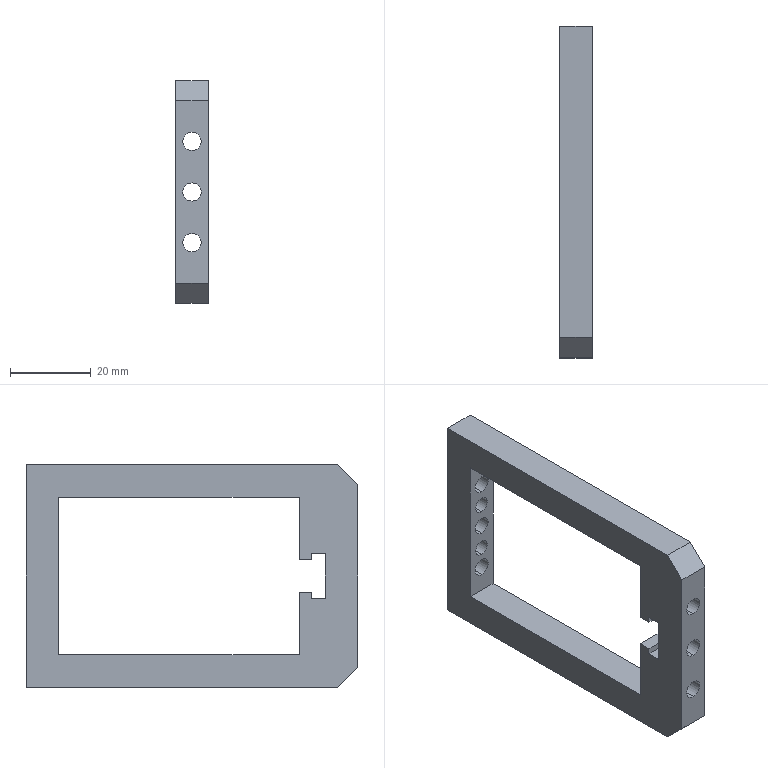Part | STEP file | 11-FG-B02211 | 1 solid | 36 faces | box 8 x 82 x 55 mm | volume 15645 mm3 | plane 20 | cylinder 16 | commonest cylinder face diameters 4.5 x12 4 x4
STEP:
#1=CARTESIAN_POINT('',(4.,74.,31.75));
#2=VERTEX_POINT('',#1);
#3=CARTESIAN_POINT('',(4.,74.,35.75));
#4=VERTEX_POINT('',#3);
#5=CARTESIAN_POINT('',(4.,74.,33.75));
#6=DIRECTION('',(0.,1.,0.));
#7=DIRECTION('',(0.,0.,1.));
#8=AXIS2_PLACEMENT_3D('',#5,#6,#7);
#9=CIRCLE('',#8,2.);
#10=EDGE_CURVE('',#2,#4,#9,.T.);
#11=ORIENTED_EDGE('',*,*,#10,.F.);
#12=CARTESIAN_POINT('',(4.,82.,31.75));
#13=VERTEX_POINT('',#12);
#14=CARTESIAN_POINT('',(4.,72.,31.75));
#15=DIRECTION('',(0.,1.,0.));
#16=VECTOR('',#15,1000.);
#17=LINE('',#14,#16);
#18=EDGE_CURVE('',#2,#13,#17,.T.);
#19=ORIENTED_EDGE('',*,*,#18,.T.);
#20=CARTESIAN_POINT('',(4.,82.,35.75));
#21=VERTEX_POINT('',#20);
#22=CARTESIAN_POINT('',(4.,82.,33.75));
#23=DIRECTION('',(0.,1.,0.));
#24=DIRECTION('',(0.,0.,1.));
#25=AXIS2_PLACEMENT_3D('',#22,#23,#24);
#26=CIRCLE('',#25,2.);
#27=EDGE_CURVE('',#13,#21,#26,.T.);
#28=ORIENTED_EDGE('',*,*,#27,.T.);
#29=CARTESIAN_POINT('',(4.,72.,35.75));
#30=DIRECTION('',(0.,1.,0.));
#31=VECTOR('',#30,1000.);
#32=LINE('',#29,#31);
#33=EDGE_CURVE('',#4,#21,#32,.T.);
#34=ORIENTED_EDGE('',*,*,#33,.F.);
#35=EDGE_LOOP('',(#11,#19,#28,#34));
#36=FACE_OUTER_BOUND('',#35,.T.);
#37=CARTESIAN_POINT('',(4.,72.,33.75));
#38=DIRECTION('',(0.,1.,0.));
#39=DIRECTION('',(0.,0.,1.));
#40=AXIS2_PLACEMENT_3D('',#37,#38,#39);
#41=CYLINDRICAL_SURFACE('',#40,2.);
#42=ADVANCED_FACE('',(#36),#41,.F.);
#43=CARTESIAN_POINT('',(4.,74.,18.839));
#44=VERTEX_POINT('',#43);
#45=CARTESIAN_POINT('',(4.,74.,22.839));
#46=VERTEX_POINT('',#45);
#47=CARTESIAN_POINT('',(4.,74.,20.839));
#48=DIRECTION('',(0.,1.,0.));
#49=DIRECTION('',(0.,0.,1.));
#50=AXIS2_PLACEMENT_3D('',#47,#48,#49);
#51=CIRCLE('',#50,2.);
#52=EDGE_CURVE('',#44,#46,#51,.T.);
#53=ORIENTED_EDGE('',*,*,#52,.F.);
#54=CARTESIAN_POINT('',(4.,82.,18.839));
#55=VERTEX_POINT('',#54);
#56=CARTESIAN_POINT('',(4.,72.,18.839));
#57=DIRECTION('',(0.,1.,0.));
#58=VECTOR('',#57,1000.);
#59=LINE('',#56,#58);
#60=EDGE_CURVE('',#44,#55,#59,.T.);
#61=ORIENTED_EDGE('',*,*,#60,.T.);
#62=CARTESIAN_POINT('',(4.,82.,22.839));
#63=VERTEX_POINT('',#62);
#64=CARTESIAN_POINT('',(4.,82.,20.839));
#65=DIRECTION('',(0.,1.,0.));
#66=DIRECTION('',(0.,0.,1.));
#67=AXIS2_PLACEMENT_3D('',#64,#65,#66);
#68=CIRCLE('',#67,2.);
#69=EDGE_CURVE('',#55,#63,#68,.T.);
#70=ORIENTED_EDGE('',*,*,#69,.T.);
#71=CARTESIAN_POINT('',(4.,72.,22.839));
#72=DIRECTION('',(0.,1.,0.));
#73=VECTOR('',#72,1000.);
#74=LINE('',#71,#73);
#75=EDGE_CURVE('',#46,#63,#74,.T.);
#76=ORIENTED_EDGE('',*,*,#75,.F.);
#77=EDGE_LOOP('',(#53,#61,#70,#76));
#78=FACE_OUTER_BOUND('',#77,.T.);
#79=CARTESIAN_POINT('',(4.,72.,20.839));
#80=DIRECTION('',(0.,1.,0.));
#81=DIRECTION('',(0.,0.,1.));
#82=AXIS2_PLACEMENT_3D('',#79,#80,#81);
#83=CYLINDRICAL_SURFACE('',#82,2.);
#84=ADVANCED_FACE('',(#78),#83,.F.);
#85=CARTESIAN_POINT('',(4.,74.,37.75));
#86=VERTEX_POINT('',#85);
#87=CARTESIAN_POINT('',(4.,74.,42.25));
#88=VERTEX_POINT('',#87);
#89=CARTESIAN_POINT('',(4.,74.,40.));
#90=DIRECTION('',(0.,1.,0.));
#91=DIRECTION('',(0.,0.,1.));
#92=AXIS2_PLACEMENT_3D('',#89,#90,#91);
#93=CIRCLE('',#92,2.25);
#94=EDGE_CURVE('',#86,#88,#93,.T.);
#95=ORIENTED_EDGE('',*,*,#94,.F.);
#96=CARTESIAN_POINT('',(4.,82.,37.75));
#97=VERTEX_POINT('',#96);
#98=CARTESIAN_POINT('',(4.,0.,37.75));
#99=DIRECTION('',(0.,1.,0.));
#100=VECTOR('',#99,1000.);
#101=LINE('',#98,#100);
#102=EDGE_CURVE('',#86,#97,#101,.T.);
#103=ORIENTED_EDGE('',*,*,#102,.T.);
#104=CARTESIAN_POINT('',(4.,82.,42.25));
#105=VERTEX_POINT('',#104);
#106=CARTESIAN_POINT('',(4.,82.,40.));
#107=DIRECTION('',(0.,1.,0.));
#108=DIRECTION('',(0.,0.,1.));
#109=AXIS2_PLACEMENT_3D('',#106,#107,#108);
#110=CIRCLE('',#109,2.25);
#111=EDGE_CURVE('',#97,#105,#110,.T.);
#112=ORIENTED_EDGE('',*,*,#111,.T.);
#113=CARTESIAN_POINT('',(4.,0.,42.25));
#114=DIRECTION('',(0.,1.,0.));
#115=VECTOR('',#114,1000.);
#116=LINE('',#113,#115);
#117=EDGE_CURVE('',#88,#105,#116,.T.);
#118=ORIENTED_EDGE('',*,*,#117,.F.);
#119=EDGE_LOOP('',(#95,#103,#112,#118));
#120=FACE_OUTER_BOUND('',#119,.T.);
#121=CARTESIAN_POINT('',(4.,0.,40.));
#122=DIRECTION('',(0.,1.,0.));
#123=DIRECTION('',(0.,0.,1.));
#124=AXIS2_PLACEMENT_3D('',#121,#122,#123);
#125=CYLINDRICAL_SURFACE('',#124,2.25);
#126=ADVANCED_FACE('',(#120),#125,.F.);
#127=CARTESIAN_POINT('',(4.,0.,37.75));
#128=VERTEX_POINT('',#127);
#129=CARTESIAN_POINT('',(4.,0.,42.25));
#130=VERTEX_POINT('',#129);
#131=CARTESIAN_POINT('',(4.,0.,40.));
#132=DIRECTION('',(0.,1.,0.));
#133=DIRECTION('',(0.,0.,1.));
#134=AXIS2_PLACEMENT_3D('',#131,#132,#133);
#135=CIRCLE('',#134,2.25);
#136=EDGE_CURVE('',#128,#130,#135,.T.);
#137=ORIENTED_EDGE('',*,*,#136,.F.);
#138=CARTESIAN_POINT('',(4.,14.5,37.75));
#139=VERTEX_POINT('',#138);
#140=CARTESIAN_POINT('',(4.,0.,37.75));
#141=DIRECTION('',(0.,1.,0.));
#142=VECTOR('',#141,1000.);
#143=LINE('',#140,#142);
#144=EDGE_CURVE('',#128,#139,#143,.T.);
#145=ORIENTED_EDGE('',*,*,#144,.T.);
#146=CARTESIAN_POINT('',(4.,14.5,42.25));
#147=VERTEX_POINT('',#146);
#148=CARTESIAN_POINT('',(4.,14.5,40.));
#149=DIRECTION('',(0.,1.,0.));
#150=DIRECTION('',(0.,0.,1.));
#151=AXIS2_PLACEMENT_3D('',#148,#149,#150);
#152=CIRCLE('',#151,2.25);
#153=EDGE_CURVE('',#139,#147,#152,.T.);
#154=ORIENTED_EDGE('',*,*,#153,.T.);
#155=CARTESIAN_POINT('',(4.,0.,42.25));
#156=DIRECTION('',(0.,1.,0.));
#157=VECTOR('',#156,1000.);
#158=LINE('',#155,#157);
#159=EDGE_CURVE('',#130,#147,#158,.T.);
#160=ORIENTED_EDGE('',*,*,#159,.F.);
#161=EDGE_LOOP('',(#137,#145,#154,#160));
#162=FACE_OUTER_BOUND('',#161,.T.);
#163=CARTESIAN_POINT('',(4.,0.,40.));
#164=DIRECTION('',(0.,1.,0.));
#165=DIRECTION('',(0.,0.,1.));
#166=AXIS2_PLACEMENT_3D('',#163,#164,#165);
#167=CYLINDRICAL_SURFACE('',#166,2.25);
#168=ADVANCED_FACE('',(#162),#167,.F.);
#169=CARTESIAN_POINT('',(4.,74.,25.25));
#170=VERTEX_POINT('',#169);
#171=CARTESIAN_POINT('',(4.,74.,29.75));
#172=VERTEX_POINT('',#171);
#173=CARTESIAN_POINT('',(4.,74.,27.5));
#174=DIRECTION('',(0.,1.,0.));
#175=DIRECTION('',(0.,0.,1.));
#176=AXIS2_PLACEMENT_3D('',#173,#174,#175);
#177=CIRCLE('',#176,2.25);
#178=EDGE_CURVE('',#170,#172,#177,.T.);
#179=ORIENTED_EDGE('',*,*,#178,.F.);
#180=CARTESIAN_POINT('',(4.,82.,25.25));
#181=VERTEX_POINT('',#180);
#182=CARTESIAN_POINT('',(4.,0.,25.25));
#183=DIRECTION('',(0.,1.,0.));
#184=VECTOR('',#183,1000.);
#185=LINE('',#182,#184);
#186=EDGE_CURVE('',#170,#181,#185,.T.);
#187=ORIENTED_EDGE('',*,*,#186,.T.);
#188=CARTESIAN_POINT('',(4.,82.,29.75));
#189=VERTEX_POINT('',#188);
#190=CARTESIAN_POINT('',(4.,82.,27.5));
#191=DIRECTION('',(0.,1.,0.));
#192=DIRECTION('',(0.,0.,1.));
#193=AXIS2_PLACEMENT_3D('',#190,#191,#192);
#194=CIRCLE('',#193,2.25);
#195=EDGE_CURVE('',#181,#189,#194,.T.);
#196=ORIENTED_EDGE('',*,*,#195,.T.);
#197=CARTESIAN_POINT('',(4.,0.,29.75));
#198=DIRECTION('',(0.,1.,0.));
#199=VECTOR('',#198,1000.);
#200=LINE('',#197,#199);
#201=EDGE_CURVE('',#172,#189,#200,.T.);
#202=ORIENTED_EDGE('',*,*,#201,.F.);
#203=EDGE_LOOP('',(#179,#187,#196,#202));
#204=FACE_OUTER_BOUND('',#203,.T.);
#205=CARTESIAN_POINT('',(4.,0.,27.5));
#206=DIRECTION('',(0.,1.,0.));
#207=DIRECTION('',(0.,0.,1.));
#208=AXIS2_PLACEMENT_3D('',#205,#206,#207);
#209=CYLINDRICAL_SURFACE('',#208,2.25);
#210=ADVANCED_FACE('',(#204),#209,.F.);
#211=CARTESIAN_POINT('',(4.,0.,25.25));
#212=VERTEX_POINT('',#211);
#213=CARTESIAN_POINT('',(4.,0.,29.75));
#214=VERTEX_POINT('',#213);
#215=CARTESIAN_POINT('',(4.,0.,27.5));
#216=DIRECTION('',(0.,1.,0.));
#217=DIRECTION('',(0.,0.,1.));
#218=AXIS2_PLACEMENT_3D('',#215,#216,#217);
#219=CIRCLE('',#218,2.25);
#220=EDGE_CURVE('',#212,#214,#219,.T.);
#221=ORIENTED_EDGE('',*,*,#220,.F.);
#222=CARTESIAN_POINT('',(4.,8.,25.25));
#223=VERTEX_POINT('',#222);
#224=CARTESIAN_POINT('',(4.,0.,25.25));
#225=DIRECTION('',(0.,1.,0.));
#226=VECTOR('',#225,1000.);
#227=LINE('',#224,#226);
#228=EDGE_CURVE('',#212,#223,#227,.T.);
#229=ORIENTED_EDGE('',*,*,#228,.T.);
#230=CARTESIAN_POINT('',(4.,8.,29.75));
#231=VERTEX_POINT('',#230);
#232=CARTESIAN_POINT('',(4.,8.,27.5));
#233=DIRECTION('',(0.,-1.,0.));
#234=DIRECTION('',(0.,0.,-1.));
#235=AXIS2_PLACEMENT_3D('',#232,#233,#234);
#236=CIRCLE('',#235,2.25);
#237=EDGE_CURVE('',#231,#223,#236,.T.);
#238=ORIENTED_EDGE('',*,*,#237,.F.);
#239=CARTESIAN_POINT('',(4.,0.,29.75));
#240=DIRECTION('',(0.,1.,0.));
#241=VECTOR('',#240,1000.);
#242=LINE('',#239,#241);
#243=EDGE_CURVE('',#214,#231,#242,.T.);
#244=ORIENTED_EDGE('',*,*,#243,.F.);
#245=EDGE_LOOP('',(#221,#229,#238,#244));
#246=FACE_OUTER_BOUND('',#245,.T.);
#247=CARTESIAN_POINT('',(4.,0.,27.5));
#248=DIRECTION('',(0.,1.,0.));
#249=DIRECTION('',(0.,0.,1.));
#250=AXIS2_PLACEMENT_3D('',#247,#248,#249);
#251=CYLINDRICAL_SURFACE('',#250,2.25);
#252=ADVANCED_FACE('',(#246),#251,.F.);
#253=CARTESIAN_POINT('',(4.,74.,12.75));
#254=VERTEX_POINT('',#253);
#255=CARTESIAN_POINT('',(4.,74.,17.25));
#256=VERTEX_POINT('',#255);
#257=CARTESIAN_POINT('',(4.,74.,15.));
#258=DIRECTION('',(0.,1.,0.));
#259=DIRECTION('',(0.,0.,1.));
#260=AXIS2_PLACEMENT_3D('',#257,#258,#259);
#261=CIRCLE('',#260,2.25);
#262=EDGE_CURVE('',#254,#256,#261,.T.);
#263=ORIENTED_EDGE('',*,*,#262,.F.);
#264=CARTESIAN_POINT('',(4.,82.,12.75));
#265=VERTEX_POINT('',#264);
#266=CARTESIAN_POINT('',(4.,0.,12.75));
#267=DIRECTION('',(0.,1.,0.));
#268=VECTOR('',#267,1000.);
#269=LINE('',#266,#268);
#270=EDGE_CURVE('',#254,#265,#269,.T.);
#271=ORIENTED_EDGE('',*,*,#270,.T.);
#272=CARTESIAN_POINT('',(4.,82.,17.25));
#273=VERTEX_POINT('',#272);
#274=CARTESIAN_POINT('',(4.,82.,15.));
#275=DIRECTION('',(0.,1.,0.));
#276=DIRECTION('',(0.,0.,1.));
#277=AXIS2_PLACEMENT_3D('',#274,#275,#276);
#278=CIRCLE('',#277,2.25);
#279=EDGE_CURVE('',#265,#273,#278,.T.);
#280=ORIENTED_EDGE('',*,*,#279,.T.);
#281=CARTESIAN_POINT('',(4.,0.,17.25));
#282=DIRECTION('',(0.,1.,0.));
#283=VECTOR('',#282,1000.);
#284=LINE('',#281,#283);
#285=EDGE_CURVE('',#256,#273,#284,.T.);
#286=ORIENTED_EDGE('',*,*,#285,.F.);
#287=EDGE_LOOP('',(#263,#271,#280,#286));
#288=FACE_OUTER_BOUND('',#287,.T.);
#289=CARTESIAN_POINT('',(4.,0.,15.));
#290=DIRECTION('',(0.,1.,0.));
#291=DIRECTION('',(0.,0.,1.));
#292=AXIS2_PLACEMENT_3D('',#289,#290,#291);
#293=CYLINDRICAL_SURFACE('',#292,2.25);
#294=ADVANCED_FACE('',(#288),#293,.F.);
#295=CARTESIAN_POINT('',(4.,0.,12.75));
#296=VERTEX_POINT('',#295);
#297=CARTESIAN_POINT('',(4.,0.,17.25));
#298=VERTEX_POINT('',#297);
#299=CARTESIAN_POINT('',(4.,0.,15.));
#300=DIRECTION('',(0.,1.,0.));
#301=DIRECTION('',(0.,0.,1.));
#302=AXIS2_PLACEMENT_3D('',#299,#300,#301);
#303=CIRCLE('',#302,2.25);
#304=EDGE_CURVE('',#296,#298,#303,.T.);
#305=ORIENTED_EDGE('',*,*,#304,.F.);
#306=CARTESIAN_POINT('',(4.,14.5,12.75));
#307=VERTEX_POINT('',#306);
#308=CARTESIAN_POINT('',(4.,0.,12.75));
#309=DIRECTION('',(0.,1.,0.));
#310=VECTOR('',#309,1000.);
#311=LINE('',#308,#310);
#312=EDGE_CURVE('',#296,#307,#311,.T.);
#313=ORIENTED_EDGE('',*,*,#312,.T.);
#314=CARTESIAN_POINT('',(4.,14.5,17.25));
#315=VERTEX_POINT('',#314);
#316=CARTESIAN_POINT('',(4.,14.5,15.));
#317=DIRECTION('',(0.,1.,0.));
#318=DIRECTION('',(0.,0.,1.));
#319=AXIS2_PLACEMENT_3D('',#316,#317,#318);
#320=CIRCLE('',#319,2.25);
#321=EDGE_CURVE('',#307,#315,#320,.T.);
#322=ORIENTED_EDGE('',*,*,#321,.T.);
#323=CARTESIAN_POINT('',(4.,0.,17.25));
#324=DIRECTION('',(0.,1.,0.));
#325=VECTOR('',#324,1000.);
#326=LINE('',#323,#325);
#327=EDGE_CURVE('',#298,#315,#326,.T.);
#328=ORIENTED_EDGE('',*,*,#327,.F.);
#329=EDGE_LOOP('',(#305,#313,#322,#328));
#330=FACE_OUTER_BOUND('',#329,.T.);
#331=CARTESIAN_POINT('',(4.,0.,15.));
#332=DIRECTION('',(0.,1.,0.));
#333=DIRECTION('',(0.,0.,1.));
#334=AXIS2_PLACEMENT_3D('',#331,#332,#333);
#335=CYLINDRICAL_SURFACE('',#334,2.25);
#336=ADVANCED_FACE('',(#330),#335,.F.);
#337=CARTESIAN_POINT('',(0.,8.,22.));
#338=VERTEX_POINT('',#337);
#339=CARTESIAN_POINT('',(0.,8.,33.));
#340=VERTEX_POINT('',#339);
#341=CARTESIAN_POINT('',(0.,8.,8.));
#342=DIRECTION('',(0.,0.,1.));
#343=VECTOR('',#342,1000.);
#344=LINE('',#341,#343);
#345=EDGE_CURVE('',#338,#340,#344,.T.);
#346=ORIENTED_EDGE('',*,*,#345,.F.);
#347=CARTESIAN_POINT('',(0.,11.5,22.));
#348=VERTEX_POINT('',#347);
#349=CARTESIAN_POINT('',(0.,11.5,22.));
#350=DIRECTION('',(0.,1.,0.));
#351=VECTOR('',#350,1000.);
#352=LINE('',#349,#351);
#353=EDGE_CURVE('',#338,#348,#352,.T.);
#354=ORIENTED_EDGE('',*,*,#353,.T.);
#355=CARTESIAN_POINT('',(0.,11.5,23.5));
#356=VERTEX_POINT('',#355);
#357=CARTESIAN_POINT('',(0.,11.5,22.));
#358=DIRECTION('',(0.,0.,1.));
#359=VECTOR('',#358,1000.);
#360=LINE('',#357,#359);
#361=EDGE_CURVE('',#348,#356,#360,.T.);
#362=ORIENTED_EDGE('',*,*,#361,.T.);
#363=CARTESIAN_POINT('',(0.,14.5,23.5));
#364=VERTEX_POINT('',#363);
#365=CARTESIAN_POINT('',(0.,11.5,23.5));
#366=DIRECTION('',(0.,1.,0.));
#367=VECTOR('',#366,1000.);
#368=LINE('',#365,#367);
#369=EDGE_CURVE('',#356,#364,#368,.T.);
#370=ORIENTED_EDGE('',*,*,#369,.T.);
#371=CARTESIAN_POINT('',(0.,14.5,8.));
#372=VERTEX_POINT('',#371);
#373=CARTESIAN_POINT('',(0.,14.5,8.));
#374=DIRECTION('',(0.,0.,-1.));
#375=VECTOR('',#374,1000.);
#376=LINE('',#373,#375);
#377=EDGE_CURVE('',#364,#372,#376,.T.);
#378=ORIENTED_EDGE('',*,*,#377,.T.);
#379=CARTESIAN_POINT('',(0.,74.,8.));
#380=VERTEX_POINT('',#379);
#381=CARTESIAN_POINT('',(0.,74.,8.));
#382=DIRECTION('',(0.,-1.,0.));
#383=VECTOR('',#382,1000.);
#384=LINE('',#381,#383);
#385=EDGE_CURVE('',#380,#372,#384,.T.);
#386=ORIENTED_EDGE('',*,*,#385,.F.);
#387=CARTESIAN_POINT('',(0.,74.,47.));
#388=VERTEX_POINT('',#387);
#389=CARTESIAN_POINT('',(0.,74.,47.));
#390=DIRECTION('',(0.,0.,-1.));
#391=VECTOR('',#390,1000.);
#392=LINE('',#389,#391);
#393=EDGE_CURVE('',#388,#380,#392,.T.);
#394=ORIENTED_EDGE('',*,*,#393,.F.);
#395=CARTESIAN_POINT('',(0.,14.5,47.));
#396=VERTEX_POINT('',#395);
#397=CARTESIAN_POINT('',(0.,8.,47.));
#398=DIRECTION('',(0.,1.,0.));
#399=VECTOR('',#398,1000.);
#400=LINE('',#397,#399);
#401=EDGE_CURVE('',#396,#388,#400,.T.);
#402=ORIENTED_EDGE('',*,*,#401,.F.);
#403=CARTESIAN_POINT('',(0.,14.5,31.5));
#404=VERTEX_POINT('',#403);
#405=CARTESIAN_POINT('',(0.,14.5,31.5));
#406=DIRECTION('',(0.,0.,-1.));
#407=VECTOR('',#406,1000.);
#408=LINE('',#405,#407);
#409=EDGE_CURVE('',#396,#404,#408,.T.);
#410=ORIENTED_EDGE('',*,*,#409,.T.);
#411=CARTESIAN_POINT('',(0.,11.5,31.5));
#412=VERTEX_POINT('',#411);
#413=CARTESIAN_POINT('',(0.,11.5,31.5));
#414=DIRECTION('',(0.,-1.,0.));
#415=VECTOR('',#414,1000.);
#416=LINE('',#413,#415);
#417=EDGE_CURVE('',#404,#412,#416,.T.);
#418=ORIENTED_EDGE('',*,*,#417,.T.);
#419=CARTESIAN_POINT('',(0.,11.5,33.));
#420=VERTEX_POINT('',#419);
#421=CARTESIAN_POINT('',(0.,11.5,31.5));
#422=DIRECTION('',(0.,0.,1.));
#423=VECTOR('',#422,1000.);
#424=LINE('',#421,#423);
#425=EDGE_CURVE('',#412,#420,#424,.T.);
#426=ORIENTED_EDGE('',*,*,#425,.T.);
#427=CARTESIAN_POINT('',(0.,11.5,33.));
#428=DIRECTION('',(0.,-1.,0.));
#429=VECTOR('',#428,1000.);
#430=LINE('',#427,#429);
#431=EDGE_CURVE('',#420,#340,#430,.T.);
#432=ORIENTED_EDGE('',*,*,#431,.T.);
#433=EDGE_LOOP('',(#346,#354,#362,#370,#378,#386,#394,#402,#410,#418,#426,#432));
#434=FACE_BOUND('',#433,.T.);
#435=CARTESIAN_POINT('',(0.,82.,0.));
#436=VERTEX_POINT('',#435);
#437=CARTESIAN_POINT('',(0.,5.,0.));
#438=VERTEX_POINT('',#437);
#439=CARTESIAN_POINT('',(0.,0.,0.));
#440=DIRECTION('',(0.,-1.,0.));
#441=VECTOR('',#440,1000.);
#442=LINE('',#439,#441);
#443=EDGE_CURVE('',#436,#438,#442,.T.);
#444=ORIENTED_EDGE('',*,*,#443,.T.);
#445=CARTESIAN_POINT('',(0.,0.,5.));
#446=VERTEX_POINT('',#445);
#447=CARTESIAN_POINT('',(0.,0.,5.));
#448=DIRECTION('',(0.,-0.7071,0.7071));
#449=VECTOR('',#448,1000.);
#450=LINE('',#447,#449);
#451=EDGE_CURVE('',#438,#446,#450,.T.);
#452=ORIENTED_EDGE('',*,*,#451,.T.);
#453=CARTESIAN_POINT('',(0.,0.,50.));
#454=VERTEX_POINT('',#453);
#455=CARTESIAN_POINT('',(0.,0.,55.));
#456=DIRECTION('',(0.,0.,-1.));
#457=VECTOR('',#456,1000.);
#458=LINE('',#455,#457);
#459=EDGE_CURVE('',#454,#446,#458,.T.);
#460=ORIENTED_EDGE('',*,*,#459,.F.);
#461=CARTESIAN_POINT('',(0.,5.,55.));
#462=VERTEX_POINT('',#461);
#463=CARTESIAN_POINT('',(0.,5.,55.));
#464=DIRECTION('',(0.,0.7071,0.7071));
#465=VECTOR('',#464,1000.);
#466=LINE('',#463,#465);
#467=EDGE_CURVE('',#454,#462,#466,.T.);
#468=ORIENTED_EDGE('',*,*,#467,.T.);
#469=CARTESIAN_POINT('',(0.,82.,55.));
#470=VERTEX_POINT('',#469);
#471=CARTESIAN_POINT('',(0.,0.,55.));
#472=DIRECTION('',(0.,-1.,0.));
#473=VECTOR('',#472,1000.);
#474=LINE('',#471,#473);
#475=EDGE_CURVE('',#470,#462,#474,.T.);
#476=ORIENTED_EDGE('',*,*,#475,.F.);
#477=CARTESIAN_POINT('',(0.,82.,55.));
#478=DIRECTION('',(0.,0.,-1.));
#479=VECTOR('',#478,1000.);
#480=LINE('',#477,#479);
#481=EDGE_CURVE('',#470,#436,#480,.T.);
#482=ORIENTED_EDGE('',*,*,#481,.T.);
#483=EDGE_LOOP('',(#444,#452,#460,#468,#476,#482));
#484=FACE_OUTER_BOUND('',#483,.T.);
#485=CARTESIAN_POINT('',(0.,0.,55.));
#486=DIRECTION('',(1.,0.,0.));
#487=DIRECTION('',(0.,0.,-1.));
#488=AXIS2_PLACEMENT_3D('',#485,#486,#487);
#489=PLANE('',#488);
#490=ADVANCED_FACE('',(#434,#484),#489,.F.);
#491=CARTESIAN_POINT('',(4.,0.,40.));
#492=DIRECTION('',(0.,1.,0.));
#493=DIRECTION('',(0.,0.,1.));
#494=AXIS2_PLACEMENT_3D('',#491,#492,#493);
#495=CIRCLE('',#494,2.25);
#496=EDGE_CURVE('',#130,#128,#495,.T.);
#497=ORIENTED_EDGE('',*,*,#496,.T.);
#498=ORIENTED_EDGE('',*,*,#136,.T.);
#499=EDGE_LOOP('',(#497,#498));
#500=FACE_BOUND('',#499,.T.);
#501=CARTESIAN_POINT('',(4.,0.,27.5));
#502=DIRECTION('',(0.,1.,0.));
#503=DIRECTION('',(0.,0.,1.));
#504=AXIS2_PLACEMENT_3D('',#501,#502,#503);
#505=CIRCLE('',#504,2.25);
#506=EDGE_CURVE('',#214,#212,#505,.T.);
#507=ORIENTED_EDGE('',*,*,#506,.T.);
#508=ORIENTED_EDGE('',*,*,#220,.T.);
#509=EDGE_LOOP('',(#507,#508));
#510=FACE_BOUND('',#509,.T.);
#511=CARTESIAN_POINT('',(4.,0.,15.));
#512=DIRECTION('',(0.,1.,0.));
#513=DIRECTION('',(0.,0.,1.));
#514=AXIS2_PLACEMENT_3D('',#511,#512,#513);
#515=CIRCLE('',#514,2.25);
#516=EDGE_CURVE('',#298,#296,#515,.T.);
#517=ORIENTED_EDGE('',*,*,#516,.T.);
#518=ORIENTED_EDGE('',*,*,#304,.T.);
#519=EDGE_LOOP('',(#517,#518));
#520=FACE_BOUND('',#519,.T.);
#521=ORIENTED_EDGE('',*,*,#459,.T.);
#522=CARTESIAN_POINT('',(8.,0.,5.));
#523=VERTEX_POINT('',#522);
#524=CARTESIAN_POINT('',(8.,0.,5.));
#525=DIRECTION('',(1.,0.,0.));
#526=VECTOR('',#525,1000.);
#527=LINE('',#524,#526);
#528=EDGE_CURVE('',#446,#523,#527,.T.);
#529=ORIENTED_EDGE('',*,*,#528,.T.);
#530=CARTESIAN_POINT('',(8.,0.,50.));
#531=VERTEX_POINT('',#530);
#532=CARTESIAN_POINT('',(8.,0.,55.));
#533=DIRECTION('',(0.,0.,-1.));
#534=VECTOR('',#533,1000.);
#535=LINE('',#532,#534);
#536=EDGE_CURVE('',#531,#523,#535,.T.);
#537=ORIENTED_EDGE('',*,*,#536,.F.);
#538=CARTESIAN_POINT('',(0.,0.,50.));
#539=DIRECTION('',(-1.,0.,0.));
#540=VECTOR('',#539,1000.);
#541=LINE('',#538,#540);
#542=EDGE_CURVE('',#531,#454,#541,.T.);
#543=ORIENTED_EDGE('',*,*,#542,.T.);
#544=EDGE_LOOP('',(#521,#529,#537,#543));
#545=FACE_OUTER_BOUND('',#544,.T.);
#546=CARTESIAN_POINT('',(0.,0.,55.));
#547=DIRECTION('',(0.,1.,0.));
#548=DIRECTION('',(0.,0.,1.));
#549=AXIS2_PLACEMENT_3D('',#546,#547,#548);
#550=PLANE('',#549);
#551=ADVANCED_FACE('',(#500,#510,#520,#545),#550,.F.);
#552=CARTESIAN_POINT('',(8.,8.,22.));
#553=VERTEX_POINT('',#552);
#554=CARTESIAN_POINT('',(8.,11.5,22.));
#555=VERTEX_POINT('',#554);
#556=CARTESIAN_POINT('',(8.,11.5,22.));
#557=DIRECTION('',(0.,1.,0.));
#558=VECTOR('',#557,1000.);
#559=LINE('',#556,#558);
#560=EDGE_CURVE('',#553,#555,#559,.T.);
#561=ORIENTED_EDGE('',*,*,#560,.F.);
#562=CARTESIAN_POINT('',(8.,8.,33.));
#563=VERTEX_POINT('',#562);
#564=CARTESIAN_POINT('',(8.,8.,8.));
#565=DIRECTION('',(0.,0.,1.));
#566=VECTOR('',#565,1000.);
#567=LINE('',#564,#566);
#568=EDGE_CURVE('',#553,#563,#567,.T.);
#569=ORIENTED_EDGE('',*,*,#568,.T.);
#570=CARTESIAN_POINT('',(8.,11.5,33.));
#571=VERTEX_POINT('',#570);
#572=CARTESIAN_POINT('',(8.,11.5,33.));
#573=DIRECTION('',(0.,-1.,0.));
#574=VECTOR('',#573,1000.);
#575=LINE('',#572,#574);
#576=EDGE_CURVE('',#571,#563,#575,.T.);
#577=ORIENTED_EDGE('',*,*,#576,.F.);
#578=CARTESIAN_POINT('',(8.,11.5,31.5));
#579=VERTEX_POINT('',#578);
#580=CARTESIAN_POINT('',(8.,11.5,31.5));
#581=DIRECTION('',(0.,0.,1.));
#582=VECTOR('',#581,1000.);
#583=LINE('',#580,#582);
#584=EDGE_CURVE('',#579,#571,#583,.T.);
#585=ORIENTED_EDGE('',*,*,#584,.F.);
#586=CARTESIAN_POINT('',(8.,14.5,31.5));
#587=VERTEX_POINT('',#586);
#588=CARTESIAN_POINT('',(8.,11.5,31.5));
#589=DIRECTION('',(0.,-1.,0.));
#590=VECTOR('',#589,1000.);
#591=LINE('',#588,#590);
#592=EDGE_CURVE('',#587,#579,#591,.T.);
#593=ORIENTED_EDGE('',*,*,#592,.F.);
#594=CARTESIAN_POINT('',(8.,14.5,47.));
#595=VERTEX_POINT('',#594);
#596=CARTESIAN_POINT('',(8.,14.5,31.5));
#597=DIRECTION('',(0.,0.,-1.));
#598=VECTOR('',#597,1000.);
#599=LINE('',#596,#598);
#600=EDGE_CURVE('',#595,#587,#599,.T.);
#601=ORIENTED_EDGE('',*,*,#600,.F.);
#602=CARTESIAN_POINT('',(8.,74.,47.));
#603=VERTEX_POINT('',#602);
#604=CARTESIAN_POINT('',(8.,8.,47.));
#605=DIRECTION('',(0.,1.,0.));
#606=VECTOR('',#605,1000.);
#607=LINE('',#604,#606);
#608=EDGE_CURVE('',#595,#603,#607,.T.);
#609=ORIENTED_EDGE('',*,*,#608,.T.);
#610=CARTESIAN_POINT('',(8.,74.,8.));
#611=VERTEX_POINT('',#610);
#612=CARTESIAN_POINT('',(8.,74.,47.));
#613=DIRECTION('',(0.,0.,-1.));
#614=VECTOR('',#613,1000.);
#615=LINE('',#612,#614);
#616=EDGE_CURVE('',#603,#611,#615,.T.);
#617=ORIENTED_EDGE('',*,*,#616,.T.);
#618=CARTESIAN_POINT('',(8.,14.5,8.));
#619=VERTEX_POINT('',#618);
#620=CARTESIAN_POINT('',(8.,74.,8.));
#621=DIRECTION('',(0.,-1.,0.));
#622=VECTOR('',#621,1000.);
#623=LINE('',#620,#622);
#624=EDGE_CURVE('',#611,#619,#623,.T.);
#625=ORIENTED_EDGE('',*,*,#624,.T.);
#626=CARTESIAN_POINT('',(8.,14.5,23.5));
#627=VERTEX_POINT('',#626);
#628=CARTESIAN_POINT('',(8.,14.5,8.));
#629=DIRECTION('',(0.,0.,-1.));
#630=VECTOR('',#629,1000.);
#631=LINE('',#628,#630);
#632=EDGE_CURVE('',#627,#619,#631,.T.);
#633=ORIENTED_EDGE('',*,*,#632,.F.);
#634=CARTESIAN_POINT('',(8.,11.5,23.5));
#635=VERTEX_POINT('',#634);
#636=CARTESIAN_POINT('',(8.,11.5,23.5));
#637=DIRECTION('',(0.,1.,0.));
#638=VECTOR('',#637,1000.);
#639=LINE('',#636,#638);
#640=EDGE_CURVE('',#635,#627,#639,.T.);
#641=ORIENTED_EDGE('',*,*,#640,.F.);
#642=CARTESIAN_POINT('',(8.,11.5,22.));
#643=DIRECTION('',(0.,0.,1.));
#644=VECTOR('',#643,1000.);
#645=LINE('',#642,#644);
#646=EDGE_CURVE('',#555,#635,#645,.T.);
#647=ORIENTED_EDGE('',*,*,#646,.F.);
#648=EDGE_LOOP('',(#561,#569,#577,#585,#593,#601,#609,#617,#625,#633,#641,#647));
#649=FACE_BOUND('',#648,.T.);
#650=ORIENTED_EDGE('',*,*,#536,.T.);
#651=CARTESIAN_POINT('',(8.,5.,0.));
#652=VERTEX_POINT('',#651);
#653=CARTESIAN_POINT('',(8.,0.,5.));
#654=DIRECTION('',(0.,0.7071,-0.7071));
#655=VECTOR('',#654,1000.);
#656=LINE('',#653,#655);
#657=EDGE_CURVE('',#523,#652,#656,.T.);
#658=ORIENTED_EDGE('',*,*,#657,.T.);
#659=CARTESIAN_POINT('',(8.,82.,0.));
#660=VERTEX_POINT('',#659);
#661=CARTESIAN_POINT('',(8.,0.,0.));
#662=DIRECTION('',(0.,1.,0.));
#663=VECTOR('',#662,1000.);
#664=LINE('',#661,#663);
#665=EDGE_CURVE('',#652,#660,#664,.T.);
#666=ORIENTED_EDGE('',*,*,#665,.T.);
#667=CARTESIAN_POINT('',(8.,82.,55.));
#668=VERTEX_POINT('',#667);
#669=CARTESIAN_POINT('',(8.,82.,55.));
#670=DIRECTION('',(0.,0.,-1.));
#671=VECTOR('',#670,1000.);
#672=LINE('',#669,#671);
#673=EDGE_CURVE('',#668,#660,#672,.T.);
#674=ORIENTED_EDGE('',*,*,#673,.F.);
#675=CARTESIAN_POINT('',(8.,5.,55.));
#676=VERTEX_POINT('',#675);
#677=CARTESIAN_POINT('',(8.,0.,55.));
#678=DIRECTION('',(0.,1.,0.));
#679=VECTOR('',#678,1000.);
#680=LINE('',#677,#679);
#681=EDGE_CURVE('',#676,#668,#680,.T.);
#682=ORIENTED_EDGE('',*,*,#681,.F.);
#683=CARTESIAN_POINT('',(8.,5.,55.));
#684=DIRECTION('',(0.,-0.7071,-0.7071));
#685=VECTOR('',#684,1000.);
#686=LINE('',#683,#685);
#687=EDGE_CURVE('',#676,#531,#686,.T.);
#688=ORIENTED_EDGE('',*,*,#687,.T.);
#689=EDGE_LOOP('',(#650,#658,#666,#674,#682,#688));
#690=FACE_OUTER_BOUND('',#689,.T.);
#691=CARTESIAN_POINT('',(8.,0.,55.));
#692=DIRECTION('',(-1.,0.,0.));
#693=DIRECTION('',(0.,0.,1.));
#694=AXIS2_PLACEMENT_3D('',#691,#692,#693);
#695=PLANE('',#694);
#696=ADVANCED_FACE('',(#649,#690),#695,.F.);
#697=CARTESIAN_POINT('',(4.,82.,33.75));
#698=DIRECTION('',(0.,1.,0.));
#699=DIRECTION('',(0.,0.,1.));
#700=AXIS2_PLACEMENT_3D('',#697,#698,#699);
#701=CIRCLE('',#700,2.);
#702=EDGE_CURVE('',#21,#13,#701,.T.);
#703=ORIENTED_EDGE('',*,*,#702,.F.);
#704=ORIENTED_EDGE('',*,*,#27,.F.);
#705=EDGE_LOOP('',(#703,#704));
#706=FACE_BOUND('',#705,.T.);
#707=CARTESIAN_POINT('',(4.,82.,20.839));
#708=DIRECTION('',(0.,1.,0.));
#709=DIRECTION('',(0.,0.,1.));
#710=AXIS2_PLACEMENT_3D('',#707,#708,#709);
#711=CIRCLE('',#710,2.);
#712=EDGE_CURVE('',#63,#55,#711,.T.);
#713=ORIENTED_EDGE('',*,*,#712,.F.);
#714=ORIENTED_EDGE('',*,*,#69,.F.);
#715=EDGE_LOOP('',(#713,#714));
#716=FACE_BOUND('',#715,.T.);
#717=CARTESIAN_POINT('',(4.,82.,40.));
#718=DIRECTION('',(0.,1.,0.));
#719=DIRECTION('',(0.,0.,1.));
#720=AXIS2_PLACEMENT_3D('',#717,#718,#719);
#721=CIRCLE('',#720,2.25);
#722=EDGE_CURVE('',#105,#97,#721,.T.);
#723=ORIENTED_EDGE('',*,*,#722,.F.);
#724=ORIENTED_EDGE('',*,*,#111,.F.);
#725=EDGE_LOOP('',(#723,#724));
#726=FACE_BOUND('',#725,.T.);
#727=CARTESIAN_POINT('',(4.,82.,27.5));
#728=DIRECTION('',(0.,1.,0.));
#729=DIRECTION('',(0.,0.,1.));
#730=AXIS2_PLACEMENT_3D('',#727,#728,#729);
#731=CIRCLE('',#730,2.25);
#732=EDGE_CURVE('',#189,#181,#731,.T.);
#733=ORIENTED_EDGE('',*,*,#732,.F.);
#734=ORIENTED_EDGE('',*,*,#195,.F.);
#735=EDGE_LOOP('',(#733,#734));
#736=FACE_BOUND('',#735,.T.);
#737=CARTESIAN_POINT('',(4.,82.,15.));
#738=DIRECTION('',(0.,1.,0.));
#739=DIRECTION('',(0.,0.,1.));
#740=AXIS2_PLACEMENT_3D('',#737,#738,#739);
#741=CIRCLE('',#740,2.25);
#742=EDGE_CURVE('',#273,#265,#741,.T.);
#743=ORIENTED_EDGE('',*,*,#742,.F.);
#744=ORIENTED_EDGE('',*,*,#279,.F.);
#745=EDGE_LOOP('',(#743,#744));
#746=FACE_BOUND('',#745,.T.);
#747=CARTESIAN_POINT('',(0.,82.,0.));
#748=DIRECTION('',(-1.,0.,0.));
#749=VECTOR('',#748,1000.);
#750=LINE('',#747,#749);
#751=EDGE_CURVE('',#660,#436,#750,.T.);
#752=ORIENTED_EDGE('',*,*,#751,.T.);
#753=ORIENTED_EDGE('',*,*,#481,.F.);
#754=CARTESIAN_POINT('',(0.,82.,55.));
#755=DIRECTION('',(-1.,0.,0.));
#756=VECTOR('',#755,1000.);
#757=LINE('',#754,#756);
#758=EDGE_CURVE('',#668,#470,#757,.T.);
#759=ORIENTED_EDGE('',*,*,#758,.F.);
#760=ORIENTED_EDGE('',*,*,#673,.T.);
#761=EDGE_LOOP('',(#752,#753,#759,#760));
#762=FACE_OUTER_BOUND('',#761,.T.);
#763=CARTESIAN_POINT('',(0.,82.,55.));
#764=DIRECTION('',(0.,-1.,0.));
#765=DIRECTION('',(0.,0.,-1.));
#766=AXIS2_PLACEMENT_3D('',#763,#764,#765);
#767=PLANE('',#766);
#768=ADVANCED_FACE('',(#706,#716,#726,#736,#746,#762),#767,.F.);
#769=ORIENTED_EDGE('',*,*,#475,.T.);
#770=CARTESIAN_POINT('',(0.,5.,55.));
#771=DIRECTION('',(1.,0.,0.));
#772=VECTOR('',#771,1000.);
#773=LINE('',#770,#772);
#774=EDGE_CURVE('',#462,#676,#773,.T.);
#775=ORIENTED_EDGE('',*,*,#774,.T.);
#776=ORIENTED_EDGE('',*,*,#681,.T.);
#777=ORIENTED_EDGE('',*,*,#758,.T.);
#778=EDGE_LOOP('',(#769,#775,#776,#777));
#779=FACE_OUTER_BOUND('',#778,.T.);
#780=CARTESIAN_POINT('',(0.,82.,55.));
#781=DIRECTION('',(0.,0.,-1.));
#782=DIRECTION('',(-1.,0.,0.));
#783=AXIS2_PLACEMENT_3D('',#780,#781,#782);
#784=PLANE('',#783);
#785=ADVANCED_FACE('',(#779),#784,.F.);
#786=ORIENTED_EDGE('',*,*,#665,.F.);
#787=CARTESIAN_POINT('',(0.,5.,0.));
#788=DIRECTION('',(-1.,0.,0.));
#789=VECTOR('',#788,1000.);
#790=LINE('',#787,#789);
#791=EDGE_CURVE('',#652,#438,#790,.T.);
#792=ORIENTED_EDGE('',*,*,#791,.T.);
#793=ORIENTED_EDGE('',*,*,#443,.F.);
#794=ORIENTED_EDGE('',*,*,#751,.F.);
#795=EDGE_LOOP('',(#786,#792,#793,#794));
#796=FACE_OUTER_BOUND('',#795,.T.);
#797=CARTESIAN_POINT('',(0.,82.,0.));
#798=DIRECTION('',(0.,0.,-1.));
#799=DIRECTION('',(-1.,0.,0.));
#800=AXIS2_PLACEMENT_3D('',#797,#798,#799);
#801=PLANE('',#800);
#802=ADVANCED_FACE('',(#796),#801,.T.);
#803=CARTESIAN_POINT('',(4.,74.,33.75));
#804=DIRECTION('',(0.,1.,0.));
#805=DIRECTION('',(0.,0.,1.));
#806=AXIS2_PLACEMENT_3D('',#803,#804,#805);
#807=CIRCLE('',#806,2.);
#808=EDGE_CURVE('',#4,#2,#807,.T.);
#809=ORIENTED_EDGE('',*,*,#808,.T.);
#810=ORIENTED_EDGE('',*,*,#10,.T.);
#811=EDGE_LOOP('',(#809,#810));
#812=FACE_BOUND('',#811,.T.);
#813=CARTESIAN_POINT('',(4.,74.,20.839));
#814=DIRECTION('',(0.,1.,0.));
#815=DIRECTION('',(0.,0.,1.));
#816=AXIS2_PLACEMENT_3D('',#813,#814,#815);
#817=CIRCLE('',#816,2.);
#818=EDGE_CURVE('',#46,#44,#817,.T.);
#819=ORIENTED_EDGE('',*,*,#818,.T.);
#820=ORIENTED_EDGE('',*,*,#52,.T.);
#821=EDGE_LOOP('',(#819,#820));
#822=FACE_BOUND('',#821,.T.);
#823=CARTESIAN_POINT('',(4.,74.,40.));
#824=DIRECTION('',(0.,1.,0.));
#825=DIRECTION('',(0.,0.,1.));
#826=AXIS2_PLACEMENT_3D('',#823,#824,#825);
#827=CIRCLE('',#826,2.25);
#828=EDGE_CURVE('',#88,#86,#827,.T.);
#829=ORIENTED_EDGE('',*,*,#828,.T.);
#830=ORIENTED_EDGE('',*,*,#94,.T.);
#831=EDGE_LOOP('',(#829,#830));
#832=FACE_BOUND('',#831,.T.);
#833=CARTESIAN_POINT('',(4.,74.,27.5));
#834=DIRECTION('',(0.,1.,0.));
#835=DIRECTION('',(0.,0.,1.));
#836=AXIS2_PLACEMENT_3D('',#833,#834,#835);
#837=CIRCLE('',#836,2.25);
#838=EDGE_CURVE('',#172,#170,#837,.T.);
#839=ORIENTED_EDGE('',*,*,#838,.T.);
#840=ORIENTED_EDGE('',*,*,#178,.T.);
#841=EDGE_LOOP('',(#839,#840));
#842=FACE_BOUND('',#841,.T.);
#843=CARTESIAN_POINT('',(4.,74.,15.));
#844=DIRECTION('',(0.,1.,0.));
#845=DIRECTION('',(0.,0.,1.));
#846=AXIS2_PLACEMENT_3D('',#843,#844,#845);
#847=CIRCLE('',#846,2.25);
#848=EDGE_CURVE('',#256,#254,#847,.T.);
#849=ORIENTED_EDGE('',*,*,#848,.T.);
#850=ORIENTED_EDGE('',*,*,#262,.T.);
#851=EDGE_LOOP('',(#849,#850));
#852=FACE_BOUND('',#851,.T.);
#853=ORIENTED_EDGE('',*,*,#393,.T.);
#854=CARTESIAN_POINT('',(8.,74.,8.));
#855=DIRECTION('',(-1.,0.,0.));
#856=VECTOR('',#855,1000.);
#857=LINE('',#854,#856);
#858=EDGE_CURVE('',#611,#380,#857,.T.);
#859=ORIENTED_EDGE('',*,*,#858,.F.);
#860=ORIENTED_EDGE('',*,*,#616,.F.);
#861=CARTESIAN_POINT('',(8.,74.,47.));
#862=DIRECTION('',(-1.,0.,0.));
#863=VECTOR('',#862,1000.);
#864=LINE('',#861,#863);
#865=EDGE_CURVE('',#603,#388,#864,.T.);
#866=ORIENTED_EDGE('',*,*,#865,.T.);
#867=EDGE_LOOP('',(#853,#859,#860,#866));
#868=FACE_OUTER_BOUND('',#867,.T.);
#869=CARTESIAN_POINT('',(8.,74.,47.));
#870=DIRECTION('',(0.,1.,0.));
#871=DIRECTION('',(0.,0.,1.));
#872=AXIS2_PLACEMENT_3D('',#869,#870,#871);
#873=PLANE('',#872);
#874=ADVANCED_FACE('',(#812,#822,#832,#842,#852,#868),#873,.F.);
#875=ORIENTED_EDGE('',*,*,#608,.F.);
#876=CARTESIAN_POINT('',(8.,14.5,47.));
#877=DIRECTION('',(-1.,0.,0.));
#878=VECTOR('',#877,1000.);
#879=LINE('',#876,#878);
#880=EDGE_CURVE('',#595,#396,#879,.T.);
#881=ORIENTED_EDGE('',*,*,#880,.T.);
#882=ORIENTED_EDGE('',*,*,#401,.T.);
#883=ORIENTED_EDGE('',*,*,#865,.F.);
#884=EDGE_LOOP('',(#875,#881,#882,#883));
#885=FACE_OUTER_BOUND('',#884,.T.);
#886=CARTESIAN_POINT('',(8.,8.,47.));
#887=DIRECTION('',(0.,0.,1.));
#888=DIRECTION('',(1.,0.,0.));
#889=AXIS2_PLACEMENT_3D('',#886,#887,#888);
#890=PLANE('',#889);
#891=ADVANCED_FACE('',(#885),#890,.F.);
#892=ORIENTED_EDGE('',*,*,#237,.T.);
#893=CARTESIAN_POINT('',(4.,8.,27.5));
#894=DIRECTION('',(0.,-1.,0.));
#895=DIRECTION('',(0.,0.,-1.));
#896=AXIS2_PLACEMENT_3D('',#893,#894,#895);
#897=CIRCLE('',#896,2.25);
#898=EDGE_CURVE('',#223,#231,#897,.T.);
#899=ORIENTED_EDGE('',*,*,#898,.T.);
#900=EDGE_LOOP('',(#892,#899));
#901=FACE_BOUND('',#900,.T.);
#902=ORIENTED_EDGE('',*,*,#568,.F.);
#903=CARTESIAN_POINT('',(8.,8.,22.));
#904=DIRECTION('',(-1.,0.,0.));
#905=VECTOR('',#904,1000.);
#906=LINE('',#903,#905);
#907=EDGE_CURVE('',#553,#338,#906,.T.);
#908=ORIENTED_EDGE('',*,*,#907,.T.);
#909=ORIENTED_EDGE('',*,*,#345,.T.);
#910=CARTESIAN_POINT('',(8.,8.,33.));
#911=DIRECTION('',(-1.,0.,0.));
#912=VECTOR('',#911,1000.);
#913=LINE('',#910,#912);
#914=EDGE_CURVE('',#563,#340,#913,.T.);
#915=ORIENTED_EDGE('',*,*,#914,.F.);
#916=EDGE_LOOP('',(#902,#908,#909,#915));
#917=FACE_OUTER_BOUND('',#916,.T.);
#918=CARTESIAN_POINT('',(8.,8.,8.));
#919=DIRECTION('',(0.,-1.,0.));
#920=DIRECTION('',(0.,0.,-1.));
#921=AXIS2_PLACEMENT_3D('',#918,#919,#920);
#922=PLANE('',#921);
#923=ADVANCED_FACE('',(#901,#917),#922,.F.);
#924=ORIENTED_EDGE('',*,*,#385,.T.);
#925=CARTESIAN_POINT('',(8.,14.5,8.));
#926=DIRECTION('',(-1.,0.,0.));
#927=VECTOR('',#926,1000.);
#928=LINE('',#925,#927);
#929=EDGE_CURVE('',#619,#372,#928,.T.);
#930=ORIENTED_EDGE('',*,*,#929,.F.);
#931=ORIENTED_EDGE('',*,*,#624,.F.);
#932=ORIENTED_EDGE('',*,*,#858,.T.);
#933=EDGE_LOOP('',(#924,#930,#931,#932));
#934=FACE_OUTER_BOUND('',#933,.T.);
#935=CARTESIAN_POINT('',(8.,74.,8.));
#936=DIRECTION('',(0.,0.,-1.));
#937=DIRECTION('',(-1.,0.,0.));
#938=AXIS2_PLACEMENT_3D('',#935,#936,#937);
#939=PLANE('',#938);
#940=ADVANCED_FACE('',(#934),#939,.F.);
#941=ORIENTED_EDGE('',*,*,#425,.F.);
#942=CARTESIAN_POINT('',(8.,11.5,31.5));
#943=DIRECTION('',(-1.,0.,0.));
#944=VECTOR('',#943,1000.);
#945=LINE('',#942,#944);
#946=EDGE_CURVE('',#579,#412,#945,.T.);
#947=ORIENTED_EDGE('',*,*,#946,.F.);
#948=ORIENTED_EDGE('',*,*,#584,.T.);
#949=CARTESIAN_POINT('',(8.,11.5,33.));
#950=DIRECTION('',(-1.,0.,0.));
#951=VECTOR('',#950,1000.);
#952=LINE('',#949,#951);
#953=EDGE_CURVE('',#571,#420,#952,.T.);
#954=ORIENTED_EDGE('',*,*,#953,.T.);
#955=EDGE_LOOP('',(#941,#947,#948,#954));
#956=FACE_OUTER_BOUND('',#955,.T.);
#957=CARTESIAN_POINT('',(8.,11.5,31.5));
#958=DIRECTION('',(0.,-1.,0.));
#959=DIRECTION('',(0.,0.,-1.));
#960=AXIS2_PLACEMENT_3D('',#957,#958,#959);
#961=PLANE('',#960);
#962=ADVANCED_FACE('',(#956),#961,.T.);
#963=ORIENTED_EDGE('',*,*,#417,.F.);
#964=CARTESIAN_POINT('',(8.,14.5,31.5));
#965=DIRECTION('',(-1.,0.,0.));
#966=VECTOR('',#965,1000.);
#967=LINE('',#964,#966);
#968=EDGE_CURVE('',#587,#404,#967,.T.);
#969=ORIENTED_EDGE('',*,*,#968,.F.);
#970=ORIENTED_EDGE('',*,*,#592,.T.);
#971=ORIENTED_EDGE('',*,*,#946,.T.);
#972=EDGE_LOOP('',(#963,#969,#970,#971));
#973=FACE_OUTER_BOUND('',#972,.T.);
#974=CARTESIAN_POINT('',(8.,11.5,31.5));
#975=DIRECTION('',(0.,0.,-1.));
#976=DIRECTION('',(0.,1.,0.));
#977=AXIS2_PLACEMENT_3D('',#974,#975,#976);
#978=PLANE('',#977);
#979=ADVANCED_FACE('',(#973),#978,.T.);
#980=CARTESIAN_POINT('',(4.,14.5,40.));
#981=DIRECTION('',(0.,1.,0.));
#982=DIRECTION('',(0.,0.,1.));
#983=AXIS2_PLACEMENT_3D('',#980,#981,#982);
#984=CIRCLE('',#983,2.25);
#985=EDGE_CURVE('',#147,#139,#984,.T.);
#986=ORIENTED_EDGE('',*,*,#985,.F.);
#987=ORIENTED_EDGE('',*,*,#153,.F.);
#988=EDGE_LOOP('',(#986,#987));
#989=FACE_BOUND('',#988,.T.);
#990=ORIENTED_EDGE('',*,*,#409,.F.);
#991=ORIENTED_EDGE('',*,*,#880,.F.);
#992=ORIENTED_EDGE('',*,*,#600,.T.);
#993=ORIENTED_EDGE('',*,*,#968,.T.);
#994=EDGE_LOOP('',(#990,#991,#992,#993));
#995=FACE_OUTER_BOUND('',#994,.T.);
#996=CARTESIAN_POINT('',(8.,14.5,31.5));
#997=DIRECTION('',(0.,1.,0.));
#998=DIRECTION('',(0.,0.,1.));
#999=AXIS2_PLACEMENT_3D('',#996,#997,#998);
#1000=PLANE('',#999);
#1001=ADVANCED_FACE('',(#989,#995),#1000,.T.);
#1002=ORIENTED_EDGE('',*,*,#431,.F.);
#1003=ORIENTED_EDGE('',*,*,#953,.F.);
#1004=ORIENTED_EDGE('',*,*,#576,.T.);
#1005=ORIENTED_EDGE('',*,*,#914,.T.);
#1006=EDGE_LOOP('',(#1002,#1003,#1004,#1005));
#1007=FACE_OUTER_BOUND('',#1006,.T.);
#1008=CARTESIAN_POINT('',(8.,11.5,33.));
#1009=DIRECTION('',(0.,0.,-1.));
#1010=DIRECTION('',(-1.,0.,0.));
#1011=AXIS2_PLACEMENT_3D('',#1008,#1009,#1010);
#1012=PLANE('',#1011);
#1013=ADVANCED_FACE('',(#1007),#1012,.T.);
#1014=CARTESIAN_POINT('',(4.,14.5,15.));
#1015=DIRECTION('',(0.,1.,0.));
#1016=DIRECTION('',(0.,0.,1.));
#1017=AXIS2_PLACEMENT_3D('',#1014,#1015,#1016);
#1018=CIRCLE('',#1017,2.25);
#1019=EDGE_CURVE('',#315,#307,#1018,.T.);
#1020=ORIENTED_EDGE('',*,*,#1019,.F.);
#1021=ORIENTED_EDGE('',*,*,#321,.F.);
#1022=EDGE_LOOP('',(#1020,#1021));
#1023=FACE_BOUND('',#1022,.T.);
#1024=ORIENTED_EDGE('',*,*,#377,.F.);
#1025=CARTESIAN_POINT('',(8.,14.5,23.5));
#1026=DIRECTION('',(-1.,0.,0.));
#1027=VECTOR('',#1026,1000.);
#1028=LINE('',#1025,#1027);
#1029=EDGE_CURVE('',#627,#364,#1028,.T.);
#1030=ORIENTED_EDGE('',*,*,#1029,.F.);
#1031=ORIENTED_EDGE('',*,*,#632,.T.);
#1032=ORIENTED_EDGE('',*,*,#929,.T.);
#1033=EDGE_LOOP('',(#1024,#1030,#1031,#1032));
#1034=FACE_OUTER_BOUND('',#1033,.T.);
#1035=CARTESIAN_POINT('',(8.,14.5,8.));
#1036=DIRECTION('',(0.,1.,0.));
#1037=DIRECTION('',(0.,0.,1.));
#1038=AXIS2_PLACEMENT_3D('',#1035,#1036,#1037);
#1039=PLANE('',#1038);
#1040=ADVANCED_FACE('',(#1023,#1034),#1039,.T.);
#1041=ORIENTED_EDGE('',*,*,#369,.F.);
#1042=CARTESIAN_POINT('',(8.,11.5,23.5));
#1043=DIRECTION('',(-1.,0.,0.));
#1044=VECTOR('',#1043,1000.);
#1045=LINE('',#1042,#1044);
#1046=EDGE_CURVE('',#635,#356,#1045,.T.);
#1047=ORIENTED_EDGE('',*,*,#1046,.F.);
#1048=ORIENTED_EDGE('',*,*,#640,.T.);
#1049=ORIENTED_EDGE('',*,*,#1029,.T.);
#1050=EDGE_LOOP('',(#1041,#1047,#1048,#1049));
#1051=FACE_OUTER_BOUND('',#1050,.T.);
#1052=CARTESIAN_POINT('',(8.,11.5,23.5));
#1053=DIRECTION('',(0.,0.,1.));
#1054=DIRECTION('',(0.,-1.,0.));
#1055=AXIS2_PLACEMENT_3D('',#1052,#1053,#1054);
#1056=PLANE('',#1055);
#1057=ADVANCED_FACE('',(#1051),#1056,.T.);
#1058=ORIENTED_EDGE('',*,*,#361,.F.);
#1059=CARTESIAN_POINT('',(8.,11.5,22.));
#1060=DIRECTION('',(-1.,0.,0.));
#1061=VECTOR('',#1060,1000.);
#1062=LINE('',#1059,#1061);
#1063=EDGE_CURVE('',#555,#348,#1062,.T.);
#1064=ORIENTED_EDGE('',*,*,#1063,.F.);
#1065=ORIENTED_EDGE('',*,*,#646,.T.);
#1066=ORIENTED_EDGE('',*,*,#1046,.T.);
#1067=EDGE_LOOP('',(#1058,#1064,#1065,#1066));
#1068=FACE_OUTER_BOUND('',#1067,.T.);
#1069=CARTESIAN_POINT('',(8.,11.5,22.));
#1070=DIRECTION('',(0.,-1.,0.));
#1071=DIRECTION('',(0.,0.,-1.));
#1072=AXIS2_PLACEMENT_3D('',#1069,#1070,#1071);
#1073=PLANE('',#1072);
#1074=ADVANCED_FACE('',(#1068),#1073,.T.);
#1075=ORIENTED_EDGE('',*,*,#353,.F.);
#1076=ORIENTED_EDGE('',*,*,#907,.F.);
#1077=ORIENTED_EDGE('',*,*,#560,.T.);
#1078=ORIENTED_EDGE('',*,*,#1063,.T.);
#1079=EDGE_LOOP('',(#1075,#1076,#1077,#1078));
#1080=FACE_OUTER_BOUND('',#1079,.T.);
#1081=CARTESIAN_POINT('',(8.,11.5,22.));
#1082=DIRECTION('',(0.,0.,1.));
#1083=DIRECTION('',(1.,0.,0.));
#1084=AXIS2_PLACEMENT_3D('',#1081,#1082,#1083);
#1085=PLANE('',#1084);
#1086=ADVANCED_FACE('',(#1080),#1085,.T.);
#1087=ORIENTED_EDGE('',*,*,#312,.F.);
#1088=ORIENTED_EDGE('',*,*,#516,.F.);
#1089=ORIENTED_EDGE('',*,*,#327,.T.);
#1090=ORIENTED_EDGE('',*,*,#1019,.T.);
#1091=EDGE_LOOP('',(#1087,#1088,#1089,#1090));
#1092=FACE_OUTER_BOUND('',#1091,.T.);
#1093=CARTESIAN_POINT('',(4.,0.,15.));
#1094=DIRECTION('',(0.,1.,0.));
#1095=DIRECTION('',(0.,0.,1.));
#1096=AXIS2_PLACEMENT_3D('',#1093,#1094,#1095);
#1097=CYLINDRICAL_SURFACE('',#1096,2.25);
#1098=ADVANCED_FACE('',(#1092),#1097,.F.);
#1099=ORIENTED_EDGE('',*,*,#270,.F.);
#1100=ORIENTED_EDGE('',*,*,#848,.F.);
#1101=ORIENTED_EDGE('',*,*,#285,.T.);
#1102=ORIENTED_EDGE('',*,*,#742,.T.);
#1103=EDGE_LOOP('',(#1099,#1100,#1101,#1102));
#1104=FACE_OUTER_BOUND('',#1103,.T.);
#1105=CARTESIAN_POINT('',(4.,0.,15.));
#1106=DIRECTION('',(0.,1.,0.));
#1107=DIRECTION('',(0.,0.,1.));
#1108=AXIS2_PLACEMENT_3D('',#1105,#1106,#1107);
#1109=CYLINDRICAL_SURFACE('',#1108,2.25);
#1110=ADVANCED_FACE('',(#1104),#1109,.F.);
#1111=ORIENTED_EDGE('',*,*,#228,.F.);
#1112=ORIENTED_EDGE('',*,*,#506,.F.);
#1113=ORIENTED_EDGE('',*,*,#243,.T.);
#1114=ORIENTED_EDGE('',*,*,#898,.F.);
#1115=EDGE_LOOP('',(#1111,#1112,#1113,#1114));
#1116=FACE_OUTER_BOUND('',#1115,.T.);
#1117=CARTESIAN_POINT('',(4.,0.,27.5));
#1118=DIRECTION('',(0.,1.,0.));
#1119=DIRECTION('',(0.,0.,1.));
#1120=AXIS2_PLACEMENT_3D('',#1117,#1118,#1119);
#1121=CYLINDRICAL_SURFACE('',#1120,2.25);
#1122=ADVANCED_FACE('',(#1116),#1121,.F.);
#1123=ORIENTED_EDGE('',*,*,#186,.F.);
#1124=ORIENTED_EDGE('',*,*,#838,.F.);
#1125=ORIENTED_EDGE('',*,*,#201,.T.);
#1126=ORIENTED_EDGE('',*,*,#732,.T.);
#1127=EDGE_LOOP('',(#1123,#1124,#1125,#1126));
#1128=FACE_OUTER_BOUND('',#1127,.T.);
#1129=CARTESIAN_POINT('',(4.,0.,27.5));
#1130=DIRECTION('',(0.,1.,0.));
#1131=DIRECTION('',(0.,0.,1.));
#1132=AXIS2_PLACEMENT_3D('',#1129,#1130,#1131);
#1133=CYLINDRICAL_SURFACE('',#1132,2.25);
#1134=ADVANCED_FACE('',(#1128),#1133,.F.);
#1135=ORIENTED_EDGE('',*,*,#144,.F.);
#1136=ORIENTED_EDGE('',*,*,#496,.F.);
#1137=ORIENTED_EDGE('',*,*,#159,.T.);
#1138=ORIENTED_EDGE('',*,*,#985,.T.);
#1139=EDGE_LOOP('',(#1135,#1136,#1137,#1138));
#1140=FACE_OUTER_BOUND('',#1139,.T.);
#1141=CARTESIAN_POINT('',(4.,0.,40.));
#1142=DIRECTION('',(0.,1.,0.));
#1143=DIRECTION('',(0.,0.,1.));
#1144=AXIS2_PLACEMENT_3D('',#1141,#1142,#1143);
#1145=CYLINDRICAL_SURFACE('',#1144,2.25);
#1146=ADVANCED_FACE('',(#1140),#1145,.F.);
#1147=ORIENTED_EDGE('',*,*,#102,.F.);
#1148=ORIENTED_EDGE('',*,*,#828,.F.);
#1149=ORIENTED_EDGE('',*,*,#117,.T.);
#1150=ORIENTED_EDGE('',*,*,#722,.T.);
#1151=EDGE_LOOP('',(#1147,#1148,#1149,#1150));
#1152=FACE_OUTER_BOUND('',#1151,.T.);
#1153=CARTESIAN_POINT('',(4.,0.,40.));
#1154=DIRECTION('',(0.,1.,0.));
#1155=DIRECTION('',(0.,0.,1.));
#1156=AXIS2_PLACEMENT_3D('',#1153,#1154,#1155);
#1157=CYLINDRICAL_SURFACE('',#1156,2.25);
#1158=ADVANCED_FACE('',(#1152),#1157,.F.);
#1159=ORIENTED_EDGE('',*,*,#60,.F.);
#1160=ORIENTED_EDGE('',*,*,#818,.F.);
#1161=ORIENTED_EDGE('',*,*,#75,.T.);
#1162=ORIENTED_EDGE('',*,*,#712,.T.);
#1163=EDGE_LOOP('',(#1159,#1160,#1161,#1162));
#1164=FACE_OUTER_BOUND('',#1163,.T.);
#1165=CARTESIAN_POINT('',(4.,72.,20.839));
#1166=DIRECTION('',(0.,1.,0.));
#1167=DIRECTION('',(0.,0.,1.));
#1168=AXIS2_PLACEMENT_3D('',#1165,#1166,#1167);
#1169=CYLINDRICAL_SURFACE('',#1168,2.);
#1170=ADVANCED_FACE('',(#1164),#1169,.F.);
#1171=ORIENTED_EDGE('',*,*,#18,.F.);
#1172=ORIENTED_EDGE('',*,*,#808,.F.);
#1173=ORIENTED_EDGE('',*,*,#33,.T.);
#1174=ORIENTED_EDGE('',*,*,#702,.T.);
#1175=EDGE_LOOP('',(#1171,#1172,#1173,#1174));
#1176=FACE_OUTER_BOUND('',#1175,.T.);
#1177=CARTESIAN_POINT('',(4.,72.,33.75));
#1178=DIRECTION('',(0.,1.,0.));
#1179=DIRECTION('',(0.,0.,1.));
#1180=AXIS2_PLACEMENT_3D('',#1177,#1178,#1179);
#1181=CYLINDRICAL_SURFACE('',#1180,2.);
#1182=ADVANCED_FACE('',(#1176),#1181,.F.);
#1183=ORIENTED_EDGE('',*,*,#451,.F.);
#1184=ORIENTED_EDGE('',*,*,#791,.F.);
#1185=ORIENTED_EDGE('',*,*,#657,.F.);
#1186=ORIENTED_EDGE('',*,*,#528,.F.);
#1187=EDGE_LOOP('',(#1183,#1184,#1185,#1186));
#1188=FACE_OUTER_BOUND('',#1187,.T.);
#1189=CARTESIAN_POINT('',(0.,0.,5.));
#1190=DIRECTION('',(0.,-0.7071,-0.7071));
#1191=DIRECTION('',(-1.,0.,0.));
#1192=AXIS2_PLACEMENT_3D('',#1189,#1190,#1191);
#1193=PLANE('',#1192);
#1194=ADVANCED_FACE('',(#1188),#1193,.T.);
#1195=ORIENTED_EDGE('',*,*,#467,.F.);
#1196=ORIENTED_EDGE('',*,*,#542,.F.);
#1197=ORIENTED_EDGE('',*,*,#687,.F.);
#1198=ORIENTED_EDGE('',*,*,#774,.F.);
#1199=EDGE_LOOP('',(#1195,#1196,#1197,#1198));
#1200=FACE_OUTER_BOUND('',#1199,.T.);
#1201=CARTESIAN_POINT('',(0.,5.,55.));
#1202=DIRECTION('',(0.,0.7071,-0.7071));
#1203=DIRECTION('',(1.,0.,0.));
#1204=AXIS2_PLACEMENT_3D('',#1201,#1202,#1203);
#1205=PLANE('',#1204);
#1206=ADVANCED_FACE('',(#1200),#1205,.F.);
#1207=CLOSED_SHELL('',(#42,#84,#126,#168,#210,#252,#294,#336,#490,#551,#696,#768,#785,#802,#874,#891,#923,#940,#962,#979,#1001,#1013,#1040,#1057,#1074,#1086,#1098,#1110,#1122,#1134,#1146,#1158,#1170,#1182,#1194,#1206));
#1208=MANIFOLD_SOLID_BREP('',#1207);
#1209=CARTESIAN_POINT('',(0.,0.,0.));
#1210=DIRECTION('',(0.,0.,1.));
#1211=DIRECTION('',(1.,0.,0.));
#1212=AXIS2_PLACEMENT_3D('',#1209,#1210,#1211);
#1213=(LENGTH_UNIT()NAMED_UNIT(*)SI_UNIT(.MILLI.,.METRE.));
#1214=UNCERTAINTY_MEASURE_WITH_UNIT(LENGTH_MEASURE(0.00001),#1213,'','');
#1215=(NAMED_UNIT(*)PLANE_ANGLE_UNIT()SI_UNIT($,.RADIAN.));
#1216=(NAMED_UNIT(*)SI_UNIT($,.STERADIAN.)SOLID_ANGLE_UNIT());
#1217=(GEOMETRIC_REPRESENTATION_CONTEXT(3)GLOBAL_UNCERTAINTY_ASSIGNED_CONTEXT((#1214))GLOBAL_UNIT_ASSIGNED_CONTEXT((#1213,#1215,#1216))REPRESENTATION_CONTEXT('',''));
#1218=ADVANCED_BREP_SHAPE_REPRESENTATION('',(#1208,#1212),#1217);